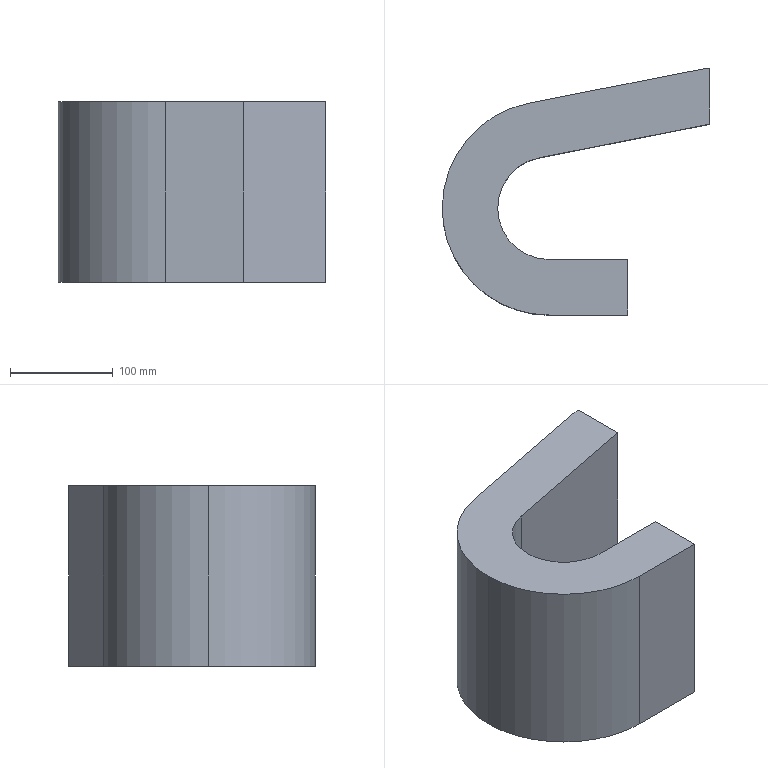Part | STEP file | TKR26H40W150R75+18L-FU-MU-Part-1 | 1 solid | 24 faces | box 260.25 x 239.7 x 176 mm | volume 1673373 mm3 | plane 16 | cylinder 8 | commonest cylinder face diameters 100 x2 114 x2 194 x2 208 x2